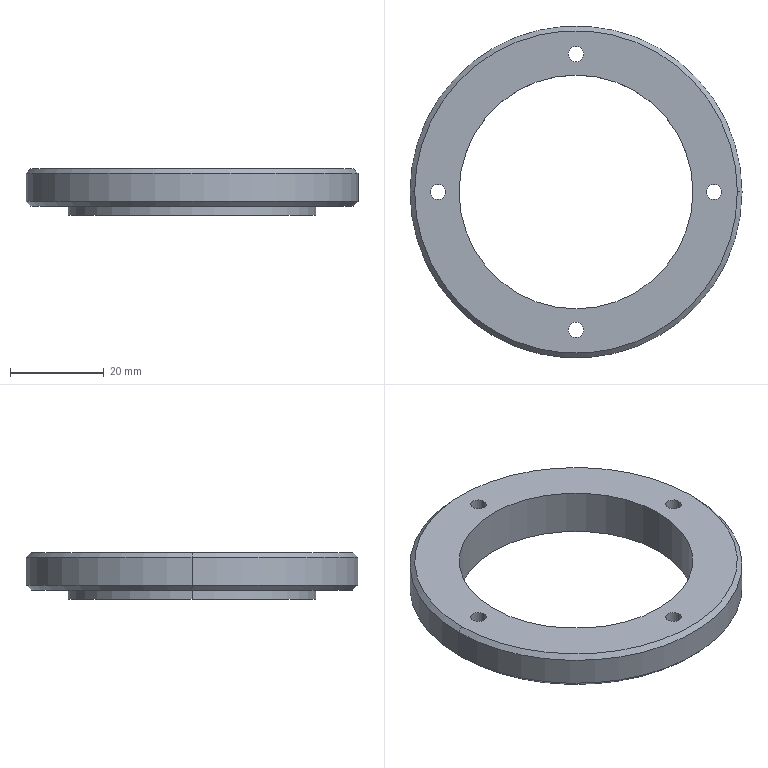Part | SolidWorks | features ICE 2, Chamfer 1, Extrusion 1, HoleWzd 1 | 1 solid | 21 faces | box 71 x 71 x 10 mm | volume 15956 mm3 | cylinder 14 | cone 4 | plane 3 | commonest cylinder face diameters 3.3 x8 50 x2 53 x2 71 x2
STEP:
#1=CARTESIAN_POINT('',(34.5,0.,10.));
#2=VERTEX_POINT('',#1);
#3=CARTESIAN_POINT('',(-34.5,0.,10.));
#4=VERTEX_POINT('',#3);
#5=CARTESIAN_POINT('',(0.,0.,10.));
#6=DIRECTION('',(0.,0.,1.));
#7=DIRECTION('',(1.,0.,0.));
#8=AXIS2_PLACEMENT_3D('',#5,#6,#7);
#9=CIRCLE('',#8,34.5);
#10=EDGE_CURVE('',#2,#4,#9,.T.);
#11=ORIENTED_EDGE('',*,*,#10,.F.);
#12=CARTESIAN_POINT('',(35.5,0.,9.));
#13=VERTEX_POINT('',#12);
#14=CARTESIAN_POINT('',(34.5,0.,10.));
#15=DIRECTION('',(0.7071,0.,-0.7071));
#16=VECTOR('',#15,1000.);
#17=LINE('',#14,#16);
#18=EDGE_CURVE('',#2,#13,#17,.T.);
#19=ORIENTED_EDGE('',*,*,#18,.T.);
#20=CARTESIAN_POINT('',(-35.5,0.,9.));
#21=VERTEX_POINT('',#20);
#22=CARTESIAN_POINT('',(0.,0.,9.));
#23=DIRECTION('',(0.,0.,-1.));
#24=DIRECTION('',(1.,0.,0.));
#25=AXIS2_PLACEMENT_3D('',#22,#23,#24);
#26=CIRCLE('',#25,35.5);
#27=EDGE_CURVE('',#21,#13,#26,.T.);
#28=ORIENTED_EDGE('',*,*,#27,.F.);
#29=CARTESIAN_POINT('',(-34.5,0.,10.));
#30=DIRECTION('',(-0.7071,0.,-0.7071));
#31=VECTOR('',#30,1000.);
#32=LINE('',#29,#31);
#33=EDGE_CURVE('',#4,#21,#32,.T.);
#34=ORIENTED_EDGE('',*,*,#33,.F.);
#35=EDGE_LOOP('',(#11,#19,#28,#34));
#36=FACE_OUTER_BOUND('',#35,.T.);
#37=CARTESIAN_POINT('',(0.,0.,10.));
#38=DIRECTION('',(0.,0.,-1.));
#39=DIRECTION('',(-1.,0.,0.));
#40=AXIS2_PLACEMENT_3D('',#37,#38,#39);
#41=CONICAL_SURFACE('',#40,34.5,0.7854);
#42=ADVANCED_FACE('',(#36),#41,.T.);
#43=CARTESIAN_POINT('',(-34.5,0.,2.));
#44=VERTEX_POINT('',#43);
#45=CARTESIAN_POINT('',(34.5,0.,2.));
#46=VERTEX_POINT('',#45);
#47=CARTESIAN_POINT('',(0.,0.,2.));
#48=DIRECTION('',(0.,0.,-1.));
#49=DIRECTION('',(-1.,0.,0.));
#50=AXIS2_PLACEMENT_3D('',#47,#48,#49);
#51=CIRCLE('',#50,34.5);
#52=EDGE_CURVE('',#44,#46,#51,.T.);
#53=ORIENTED_EDGE('',*,*,#52,.F.);
#54=CARTESIAN_POINT('',(-35.5,0.,3.));
#55=VERTEX_POINT('',#54);
#56=CARTESIAN_POINT('',(-34.5,0.,2.));
#57=DIRECTION('',(-0.7071,0.,0.7071));
#58=VECTOR('',#57,1000.);
#59=LINE('',#56,#58);
#60=EDGE_CURVE('',#44,#55,#59,.T.);
#61=ORIENTED_EDGE('',*,*,#60,.T.);
#62=CARTESIAN_POINT('',(35.5,0.,3.));
#63=VERTEX_POINT('',#62);
#64=CARTESIAN_POINT('',(0.,0.,3.));
#65=DIRECTION('',(0.,0.,1.));
#66=DIRECTION('',(-1.,0.,0.));
#67=AXIS2_PLACEMENT_3D('',#64,#65,#66);
#68=CIRCLE('',#67,35.5);
#69=EDGE_CURVE('',#63,#55,#68,.T.);
#70=ORIENTED_EDGE('',*,*,#69,.F.);
#71=CARTESIAN_POINT('',(34.5,0.,2.));
#72=DIRECTION('',(0.7071,0.,0.7071));
#73=VECTOR('',#72,1000.);
#74=LINE('',#71,#73);
#75=EDGE_CURVE('',#46,#63,#74,.T.);
#76=ORIENTED_EDGE('',*,*,#75,.F.);
#77=EDGE_LOOP('',(#53,#61,#70,#76));
#78=FACE_OUTER_BOUND('',#77,.T.);
#79=CARTESIAN_POINT('',(0.,0.,2.));
#80=DIRECTION('',(0.,0.,1.));
#81=DIRECTION('',(1.,0.,0.));
#82=AXIS2_PLACEMENT_3D('',#79,#80,#81);
#83=CONICAL_SURFACE('',#82,34.5,0.7854);
#84=ADVANCED_FACE('',(#78),#83,.T.);
#85=CARTESIAN_POINT('',(1.65,-29.5,2.));
#86=VERTEX_POINT('',#85);
#87=CARTESIAN_POINT('',(-1.65,-29.5,2.));
#88=VERTEX_POINT('',#87);
#89=CARTESIAN_POINT('',(0.,-29.5,2.));
#90=DIRECTION('',(0.,0.,-1.));
#91=DIRECTION('',(-1.,0.,0.));
#92=AXIS2_PLACEMENT_3D('',#89,#90,#91);
#93=CIRCLE('',#92,1.65);
#94=EDGE_CURVE('',#86,#88,#93,.T.);
#95=ORIENTED_EDGE('',*,*,#94,.T.);
#96=CARTESIAN_POINT('',(-1.65,-29.5,10.));
#97=VERTEX_POINT('',#96);
#98=CARTESIAN_POINT('',(-1.65,-29.5,10.));
#99=DIRECTION('',(0.,0.,1.));
#100=VECTOR('',#99,1000.);
#101=LINE('',#98,#100);
#102=EDGE_CURVE('',#88,#97,#101,.T.);
#103=ORIENTED_EDGE('',*,*,#102,.T.);
#104=CARTESIAN_POINT('',(1.65,-29.5,10.));
#105=VERTEX_POINT('',#104);
#106=CARTESIAN_POINT('',(0.,-29.5,10.));
#107=DIRECTION('',(0.,0.,1.));
#108=DIRECTION('',(1.,0.,0.));
#109=AXIS2_PLACEMENT_3D('',#106,#107,#108);
#110=CIRCLE('',#109,1.65);
#111=EDGE_CURVE('',#97,#105,#110,.T.);
#112=ORIENTED_EDGE('',*,*,#111,.T.);
#113=CARTESIAN_POINT('',(1.65,-29.5,10.));
#114=DIRECTION('',(0.,0.,1.));
#115=VECTOR('',#114,1000.);
#116=LINE('',#113,#115);
#117=EDGE_CURVE('',#86,#105,#116,.T.);
#118=ORIENTED_EDGE('',*,*,#117,.F.);
#119=EDGE_LOOP('',(#95,#103,#112,#118));
#120=FACE_OUTER_BOUND('',#119,.T.);
#121=CARTESIAN_POINT('',(0.,-29.5,10.));
#122=DIRECTION('',(0.,0.,1.));
#123=DIRECTION('',(1.,0.,0.));
#124=AXIS2_PLACEMENT_3D('',#121,#122,#123);
#125=CYLINDRICAL_SURFACE('',#124,1.65);
#126=ADVANCED_FACE('',(#120),#125,.F.);
#127=CARTESIAN_POINT('',(-27.85,0.,2.));
#128=VERTEX_POINT('',#127);
#129=CARTESIAN_POINT('',(-31.15,0.,2.));
#130=VERTEX_POINT('',#129);
#131=CARTESIAN_POINT('',(-29.5,0.,2.));
#132=DIRECTION('',(0.,0.,-1.));
#133=DIRECTION('',(-1.,0.,0.));
#134=AXIS2_PLACEMENT_3D('',#131,#132,#133);
#135=CIRCLE('',#134,1.65);
#136=EDGE_CURVE('',#128,#130,#135,.T.);
#137=ORIENTED_EDGE('',*,*,#136,.T.);
#138=CARTESIAN_POINT('',(-31.15,0.,10.));
#139=VERTEX_POINT('',#138);
#140=CARTESIAN_POINT('',(-31.15,0.,10.));
#141=DIRECTION('',(0.,0.,1.));
#142=VECTOR('',#141,1000.);
#143=LINE('',#140,#142);
#144=EDGE_CURVE('',#130,#139,#143,.T.);
#145=ORIENTED_EDGE('',*,*,#144,.T.);
#146=CARTESIAN_POINT('',(-27.85,0.,10.));
#147=VERTEX_POINT('',#146);
#148=CARTESIAN_POINT('',(-29.5,0.,10.));
#149=DIRECTION('',(0.,0.,1.));
#150=DIRECTION('',(1.,0.,0.));
#151=AXIS2_PLACEMENT_3D('',#148,#149,#150);
#152=CIRCLE('',#151,1.65);
#153=EDGE_CURVE('',#139,#147,#152,.T.);
#154=ORIENTED_EDGE('',*,*,#153,.T.);
#155=CARTESIAN_POINT('',(-27.85,0.,10.));
#156=DIRECTION('',(0.,0.,1.));
#157=VECTOR('',#156,1000.);
#158=LINE('',#155,#157);
#159=EDGE_CURVE('',#128,#147,#158,.T.);
#160=ORIENTED_EDGE('',*,*,#159,.F.);
#161=EDGE_LOOP('',(#137,#145,#154,#160));
#162=FACE_OUTER_BOUND('',#161,.T.);
#163=CARTESIAN_POINT('',(-29.5,0.,10.));
#164=DIRECTION('',(0.,0.,1.));
#165=DIRECTION('',(1.,0.,0.));
#166=AXIS2_PLACEMENT_3D('',#163,#164,#165);
#167=CYLINDRICAL_SURFACE('',#166,1.65);
#168=ADVANCED_FACE('',(#162),#167,.F.);
#169=CARTESIAN_POINT('',(1.65,29.5,2.));
#170=VERTEX_POINT('',#169);
#171=CARTESIAN_POINT('',(-1.65,29.5,2.));
#172=VERTEX_POINT('',#171);
#173=CARTESIAN_POINT('',(0.,29.5,2.));
#174=DIRECTION('',(0.,0.,-1.));
#175=DIRECTION('',(-1.,0.,0.));
#176=AXIS2_PLACEMENT_3D('',#173,#174,#175);
#177=CIRCLE('',#176,1.65);
#178=EDGE_CURVE('',#170,#172,#177,.T.);
#179=ORIENTED_EDGE('',*,*,#178,.T.);
#180=CARTESIAN_POINT('',(-1.65,29.5,10.));
#181=VERTEX_POINT('',#180);
#182=CARTESIAN_POINT('',(-1.65,29.5,10.));
#183=DIRECTION('',(0.,0.,1.));
#184=VECTOR('',#183,1000.);
#185=LINE('',#182,#184);
#186=EDGE_CURVE('',#172,#181,#185,.T.);
#187=ORIENTED_EDGE('',*,*,#186,.T.);
#188=CARTESIAN_POINT('',(1.65,29.5,10.));
#189=VERTEX_POINT('',#188);
#190=CARTESIAN_POINT('',(0.,29.5,10.));
#191=DIRECTION('',(0.,0.,1.));
#192=DIRECTION('',(1.,0.,0.));
#193=AXIS2_PLACEMENT_3D('',#190,#191,#192);
#194=CIRCLE('',#193,1.65);
#195=EDGE_CURVE('',#181,#189,#194,.T.);
#196=ORIENTED_EDGE('',*,*,#195,.T.);
#197=CARTESIAN_POINT('',(1.65,29.5,10.));
#198=DIRECTION('',(0.,0.,1.));
#199=VECTOR('',#198,1000.);
#200=LINE('',#197,#199);
#201=EDGE_CURVE('',#170,#189,#200,.T.);
#202=ORIENTED_EDGE('',*,*,#201,.F.);
#203=EDGE_LOOP('',(#179,#187,#196,#202));
#204=FACE_OUTER_BOUND('',#203,.T.);
#205=CARTESIAN_POINT('',(0.,29.5,10.));
#206=DIRECTION('',(0.,0.,1.));
#207=DIRECTION('',(1.,0.,0.));
#208=AXIS2_PLACEMENT_3D('',#205,#206,#207);
#209=CYLINDRICAL_SURFACE('',#208,1.65);
#210=ADVANCED_FACE('',(#204),#209,.F.);
#211=CARTESIAN_POINT('',(31.15,0.,2.));
#212=VERTEX_POINT('',#211);
#213=CARTESIAN_POINT('',(27.85,0.,2.));
#214=VERTEX_POINT('',#213);
#215=CARTESIAN_POINT('',(29.5,0.,2.));
#216=DIRECTION('',(0.,0.,-1.));
#217=DIRECTION('',(-1.,0.,0.));
#218=AXIS2_PLACEMENT_3D('',#215,#216,#217);
#219=CIRCLE('',#218,1.65);
#220=EDGE_CURVE('',#212,#214,#219,.T.);
#221=ORIENTED_EDGE('',*,*,#220,.T.);
#222=CARTESIAN_POINT('',(27.85,0.,10.));
#223=VERTEX_POINT('',#222);
#224=CARTESIAN_POINT('',(27.85,0.,10.));
#225=DIRECTION('',(0.,0.,1.));
#226=VECTOR('',#225,1000.);
#227=LINE('',#224,#226);
#228=EDGE_CURVE('',#214,#223,#227,.T.);
#229=ORIENTED_EDGE('',*,*,#228,.T.);
#230=CARTESIAN_POINT('',(31.15,0.,10.));
#231=VERTEX_POINT('',#230);
#232=CARTESIAN_POINT('',(29.5,0.,10.));
#233=DIRECTION('',(0.,0.,1.));
#234=DIRECTION('',(1.,0.,0.));
#235=AXIS2_PLACEMENT_3D('',#232,#233,#234);
#236=CIRCLE('',#235,1.65);
#237=EDGE_CURVE('',#223,#231,#236,.T.);
#238=ORIENTED_EDGE('',*,*,#237,.T.);
#239=CARTESIAN_POINT('',(31.15,0.,10.));
#240=DIRECTION('',(0.,0.,1.));
#241=VECTOR('',#240,1000.);
#242=LINE('',#239,#241);
#243=EDGE_CURVE('',#212,#231,#242,.T.);
#244=ORIENTED_EDGE('',*,*,#243,.F.);
#245=EDGE_LOOP('',(#221,#229,#238,#244));
#246=FACE_OUTER_BOUND('',#245,.T.);
#247=CARTESIAN_POINT('',(29.5,0.,10.));
#248=DIRECTION('',(0.,0.,1.));
#249=DIRECTION('',(1.,0.,0.));
#250=AXIS2_PLACEMENT_3D('',#247,#248,#249);
#251=CYLINDRICAL_SURFACE('',#250,1.65);
#252=ADVANCED_FACE('',(#246),#251,.F.);
#253=CARTESIAN_POINT('',(-26.5,0.,2.));
#254=VERTEX_POINT('',#253);
#255=CARTESIAN_POINT('',(26.5,0.,2.));
#256=VERTEX_POINT('',#255);
#257=CARTESIAN_POINT('',(0.,0.,2.));
#258=DIRECTION('',(0.,0.,-1.));
#259=DIRECTION('',(-1.,0.,0.));
#260=AXIS2_PLACEMENT_3D('',#257,#258,#259);
#261=CIRCLE('',#260,26.5);
#262=EDGE_CURVE('',#254,#256,#261,.T.);
#263=ORIENTED_EDGE('',*,*,#262,.T.);
#264=CARTESIAN_POINT('',(26.5,0.,0.));
#265=VERTEX_POINT('',#264);
#266=CARTESIAN_POINT('',(26.5,0.,2.));
#267=DIRECTION('',(0.,0.,-1.));
#268=VECTOR('',#267,1000.);
#269=LINE('',#266,#268);
#270=EDGE_CURVE('',#256,#265,#269,.T.);
#271=ORIENTED_EDGE('',*,*,#270,.T.);
#272=CARTESIAN_POINT('',(-26.5,0.,0.));
#273=VERTEX_POINT('',#272);
#274=CARTESIAN_POINT('',(0.,0.,0.));
#275=DIRECTION('',(0.,0.,-1.));
#276=DIRECTION('',(-1.,0.,0.));
#277=AXIS2_PLACEMENT_3D('',#274,#275,#276);
#278=CIRCLE('',#277,26.5);
#279=EDGE_CURVE('',#273,#265,#278,.T.);
#280=ORIENTED_EDGE('',*,*,#279,.F.);
#281=CARTESIAN_POINT('',(-26.5,0.,2.));
#282=DIRECTION('',(0.,0.,-1.));
#283=VECTOR('',#282,1000.);
#284=LINE('',#281,#283);
#285=EDGE_CURVE('',#254,#273,#284,.T.);
#286=ORIENTED_EDGE('',*,*,#285,.F.);
#287=EDGE_LOOP('',(#263,#271,#280,#286));
#288=FACE_OUTER_BOUND('',#287,.T.);
#289=CARTESIAN_POINT('',(0.,0.,2.));
#290=DIRECTION('',(0.,0.,-1.));
#291=DIRECTION('',(-1.,0.,0.));
#292=AXIS2_PLACEMENT_3D('',#289,#290,#291);
#293=CYLINDRICAL_SURFACE('',#292,26.5);
#294=ADVANCED_FACE('',(#288),#293,.T.);
#295=CARTESIAN_POINT('',(-25.,0.,10.));
#296=VERTEX_POINT('',#295);
#297=CARTESIAN_POINT('',(25.,0.,10.));
#298=VERTEX_POINT('',#297);
#299=CARTESIAN_POINT('',(0.,0.,10.));
#300=DIRECTION('',(0.,0.,1.));
#301=DIRECTION('',(1.,0.,0.));
#302=AXIS2_PLACEMENT_3D('',#299,#300,#301);
#303=CIRCLE('',#302,25.);
#304=EDGE_CURVE('',#296,#298,#303,.T.);
#305=ORIENTED_EDGE('',*,*,#304,.T.);
#306=CARTESIAN_POINT('',(25.,0.,0.));
#307=VERTEX_POINT('',#306);
#308=CARTESIAN_POINT('',(25.,0.,10.));
#309=DIRECTION('',(0.,0.,-1.));
#310=VECTOR('',#309,1000.);
#311=LINE('',#308,#310);
#312=EDGE_CURVE('',#298,#307,#311,.T.);
#313=ORIENTED_EDGE('',*,*,#312,.T.);
#314=CARTESIAN_POINT('',(-25.,0.,0.));
#315=VERTEX_POINT('',#314);
#316=CARTESIAN_POINT('',(0.,0.,0.));
#317=DIRECTION('',(0.,0.,1.));
#318=DIRECTION('',(1.,0.,0.));
#319=AXIS2_PLACEMENT_3D('',#316,#317,#318);
#320=CIRCLE('',#319,25.);
#321=EDGE_CURVE('',#315,#307,#320,.T.);
#322=ORIENTED_EDGE('',*,*,#321,.F.);
#323=CARTESIAN_POINT('',(-25.,0.,10.));
#324=DIRECTION('',(0.,0.,-1.));
#325=VECTOR('',#324,1000.);
#326=LINE('',#323,#325);
#327=EDGE_CURVE('',#296,#315,#326,.T.);
#328=ORIENTED_EDGE('',*,*,#327,.F.);
#329=EDGE_LOOP('',(#305,#313,#322,#328));
#330=FACE_OUTER_BOUND('',#329,.T.);
#331=CARTESIAN_POINT('',(0.,0.,10.));
#332=DIRECTION('',(0.,0.,-1.));
#333=DIRECTION('',(-1.,0.,0.));
#334=AXIS2_PLACEMENT_3D('',#331,#332,#333);
#335=CYLINDRICAL_SURFACE('',#334,25.);
#336=ADVANCED_FACE('',(#330),#335,.F.);
#337=ORIENTED_EDGE('',*,*,#27,.T.);
#338=CARTESIAN_POINT('',(35.5,0.,10.));
#339=DIRECTION('',(0.,0.,-1.));
#340=VECTOR('',#339,1000.);
#341=LINE('',#338,#340);
#342=EDGE_CURVE('',#13,#63,#341,.T.);
#343=ORIENTED_EDGE('',*,*,#342,.T.);
#344=ORIENTED_EDGE('',*,*,#69,.T.);
#345=CARTESIAN_POINT('',(-35.5,0.,10.));
#346=DIRECTION('',(0.,0.,-1.));
#347=VECTOR('',#346,1000.);
#348=LINE('',#345,#347);
#349=EDGE_CURVE('',#21,#55,#348,.T.);
#350=ORIENTED_EDGE('',*,*,#349,.F.);
#351=EDGE_LOOP('',(#337,#343,#344,#350));
#352=FACE_OUTER_BOUND('',#351,.T.);
#353=CARTESIAN_POINT('',(0.,0.,10.));
#354=DIRECTION('',(0.,0.,-1.));
#355=DIRECTION('',(-1.,0.,0.));
#356=AXIS2_PLACEMENT_3D('',#353,#354,#355);
#357=CYLINDRICAL_SURFACE('',#356,35.5);
#358=ADVANCED_FACE('',(#352),#357,.T.);
#359=ORIENTED_EDGE('',*,*,#321,.T.);
#360=CARTESIAN_POINT('',(0.,0.,0.));
#361=DIRECTION('',(0.,0.,1.));
#362=DIRECTION('',(1.,0.,0.));
#363=AXIS2_PLACEMENT_3D('',#360,#361,#362);
#364=CIRCLE('',#363,25.);
#365=EDGE_CURVE('',#307,#315,#364,.T.);
#366=ORIENTED_EDGE('',*,*,#365,.T.);
#367=EDGE_LOOP('',(#359,#366));
#368=FACE_BOUND('',#367,.T.);
#369=ORIENTED_EDGE('',*,*,#279,.T.);
#370=CARTESIAN_POINT('',(0.,0.,0.));
#371=DIRECTION('',(0.,0.,-1.));
#372=DIRECTION('',(-1.,0.,0.));
#373=AXIS2_PLACEMENT_3D('',#370,#371,#372);
#374=CIRCLE('',#373,26.5);
#375=EDGE_CURVE('',#265,#273,#374,.T.);
#376=ORIENTED_EDGE('',*,*,#375,.T.);
#377=EDGE_LOOP('',(#369,#376));
#378=FACE_OUTER_BOUND('',#377,.T.);
#379=CARTESIAN_POINT('',(0.,0.,0.));
#380=DIRECTION('',(0.,0.,1.));
#381=DIRECTION('',(1.,0.,0.));
#382=AXIS2_PLACEMENT_3D('',#379,#380,#381);
#383=PLANE('',#382);
#384=ADVANCED_FACE('',(#368,#378),#383,.F.);
#385=ORIENTED_EDGE('',*,*,#342,.F.);
#386=CARTESIAN_POINT('',(0.,0.,9.));
#387=DIRECTION('',(0.,0.,-1.));
#388=DIRECTION('',(1.,0.,0.));
#389=AXIS2_PLACEMENT_3D('',#386,#387,#388);
#390=CIRCLE('',#389,35.5);
#391=EDGE_CURVE('',#13,#21,#390,.T.);
#392=ORIENTED_EDGE('',*,*,#391,.T.);
#393=ORIENTED_EDGE('',*,*,#349,.T.);
#394=CARTESIAN_POINT('',(0.,0.,3.));
#395=DIRECTION('',(0.,0.,1.));
#396=DIRECTION('',(-1.,0.,0.));
#397=AXIS2_PLACEMENT_3D('',#394,#395,#396);
#398=CIRCLE('',#397,35.5);
#399=EDGE_CURVE('',#55,#63,#398,.T.);
#400=ORIENTED_EDGE('',*,*,#399,.T.);
#401=EDGE_LOOP('',(#385,#392,#393,#400));
#402=FACE_OUTER_BOUND('',#401,.T.);
#403=CARTESIAN_POINT('',(0.,0.,10.));
#404=DIRECTION('',(0.,0.,-1.));
#405=DIRECTION('',(-1.,0.,0.));
#406=AXIS2_PLACEMENT_3D('',#403,#404,#405);
#407=CYLINDRICAL_SURFACE('',#406,35.5);
#408=ADVANCED_FACE('',(#402),#407,.T.);
#409=CARTESIAN_POINT('',(0.,0.,10.));
#410=DIRECTION('',(0.,0.,1.));
#411=DIRECTION('',(1.,0.,0.));
#412=AXIS2_PLACEMENT_3D('',#409,#410,#411);
#413=CIRCLE('',#412,34.5);
#414=EDGE_CURVE('',#4,#2,#413,.T.);
#415=ORIENTED_EDGE('',*,*,#414,.T.);
#416=ORIENTED_EDGE('',*,*,#10,.T.);
#417=EDGE_LOOP('',(#415,#416));
#418=FACE_OUTER_BOUND('',#417,.T.);
#419=CARTESIAN_POINT('',(0.,-29.5,10.));
#420=DIRECTION('',(0.,0.,1.));
#421=DIRECTION('',(1.,0.,0.));
#422=AXIS2_PLACEMENT_3D('',#419,#420,#421);
#423=CIRCLE('',#422,1.65);
#424=EDGE_CURVE('',#105,#97,#423,.T.);
#425=ORIENTED_EDGE('',*,*,#424,.F.);
#426=ORIENTED_EDGE('',*,*,#111,.F.);
#427=EDGE_LOOP('',(#425,#426));
#428=FACE_BOUND('',#427,.T.);
#429=CARTESIAN_POINT('',(-29.5,0.,10.));
#430=DIRECTION('',(0.,0.,1.));
#431=DIRECTION('',(1.,0.,0.));
#432=AXIS2_PLACEMENT_3D('',#429,#430,#431);
#433=CIRCLE('',#432,1.65);
#434=EDGE_CURVE('',#147,#139,#433,.T.);
#435=ORIENTED_EDGE('',*,*,#434,.F.);
#436=ORIENTED_EDGE('',*,*,#153,.F.);
#437=EDGE_LOOP('',(#435,#436));
#438=FACE_BOUND('',#437,.T.);
#439=CARTESIAN_POINT('',(0.,29.5,10.));
#440=DIRECTION('',(0.,0.,1.));
#441=DIRECTION('',(1.,0.,0.));
#442=AXIS2_PLACEMENT_3D('',#439,#440,#441);
#443=CIRCLE('',#442,1.65);
#444=EDGE_CURVE('',#189,#181,#443,.T.);
#445=ORIENTED_EDGE('',*,*,#444,.F.);
#446=ORIENTED_EDGE('',*,*,#195,.F.);
#447=EDGE_LOOP('',(#445,#446));
#448=FACE_BOUND('',#447,.T.);
#449=CARTESIAN_POINT('',(29.5,0.,10.));
#450=DIRECTION('',(0.,0.,1.));
#451=DIRECTION('',(1.,0.,0.));
#452=AXIS2_PLACEMENT_3D('',#449,#450,#451);
#453=CIRCLE('',#452,1.65);
#454=EDGE_CURVE('',#231,#223,#453,.T.);
#455=ORIENTED_EDGE('',*,*,#454,.F.);
#456=ORIENTED_EDGE('',*,*,#237,.F.);
#457=EDGE_LOOP('',(#455,#456));
#458=FACE_BOUND('',#457,.T.);
#459=ORIENTED_EDGE('',*,*,#304,.F.);
#460=CARTESIAN_POINT('',(0.,0.,10.));
#461=DIRECTION('',(0.,0.,1.));
#462=DIRECTION('',(1.,0.,0.));
#463=AXIS2_PLACEMENT_3D('',#460,#461,#462);
#464=CIRCLE('',#463,25.);
#465=EDGE_CURVE('',#298,#296,#464,.T.);
#466=ORIENTED_EDGE('',*,*,#465,.F.);
#467=EDGE_LOOP('',(#459,#466));
#468=FACE_BOUND('',#467,.T.);
#469=CARTESIAN_POINT('',(0.,0.,10.));
#470=DIRECTION('',(0.,0.,1.));
#471=DIRECTION('',(1.,0.,0.));
#472=AXIS2_PLACEMENT_3D('',#469,#470,#471);
#473=PLANE('',#472);
#474=ADVANCED_FACE('',(#418,#428,#438,#448,#458,#468),#473,.T.);
#475=ORIENTED_EDGE('',*,*,#312,.F.);
#476=ORIENTED_EDGE('',*,*,#465,.T.);
#477=ORIENTED_EDGE('',*,*,#327,.T.);
#478=ORIENTED_EDGE('',*,*,#365,.F.);
#479=EDGE_LOOP('',(#475,#476,#477,#478));
#480=FACE_OUTER_BOUND('',#479,.T.);
#481=CARTESIAN_POINT('',(0.,0.,10.));
#482=DIRECTION('',(0.,0.,-1.));
#483=DIRECTION('',(-1.,0.,0.));
#484=AXIS2_PLACEMENT_3D('',#481,#482,#483);
#485=CYLINDRICAL_SURFACE('',#484,25.);
#486=ADVANCED_FACE('',(#480),#485,.F.);
#487=CARTESIAN_POINT('',(0.,0.,2.));
#488=DIRECTION('',(0.,0.,-1.));
#489=DIRECTION('',(-1.,0.,0.));
#490=AXIS2_PLACEMENT_3D('',#487,#488,#489);
#491=CIRCLE('',#490,34.5);
#492=EDGE_CURVE('',#46,#44,#491,.T.);
#493=ORIENTED_EDGE('',*,*,#492,.T.);
#494=ORIENTED_EDGE('',*,*,#52,.T.);
#495=EDGE_LOOP('',(#493,#494));
#496=FACE_OUTER_BOUND('',#495,.T.);
#497=ORIENTED_EDGE('',*,*,#94,.F.);
#498=CARTESIAN_POINT('',(0.,-29.5,2.));
#499=DIRECTION('',(0.,0.,-1.));
#500=DIRECTION('',(-1.,0.,0.));
#501=AXIS2_PLACEMENT_3D('',#498,#499,#500);
#502=CIRCLE('',#501,1.65);
#503=EDGE_CURVE('',#88,#86,#502,.T.);
#504=ORIENTED_EDGE('',*,*,#503,.F.);
#505=EDGE_LOOP('',(#497,#504));
#506=FACE_BOUND('',#505,.T.);
#507=ORIENTED_EDGE('',*,*,#136,.F.);
#508=CARTESIAN_POINT('',(-29.5,0.,2.));
#509=DIRECTION('',(0.,0.,-1.));
#510=DIRECTION('',(-1.,0.,0.));
#511=AXIS2_PLACEMENT_3D('',#508,#509,#510);
#512=CIRCLE('',#511,1.65);
#513=EDGE_CURVE('',#130,#128,#512,.T.);
#514=ORIENTED_EDGE('',*,*,#513,.F.);
#515=EDGE_LOOP('',(#507,#514));
#516=FACE_BOUND('',#515,.T.);
#517=ORIENTED_EDGE('',*,*,#178,.F.);
#518=CARTESIAN_POINT('',(0.,29.5,2.));
#519=DIRECTION('',(0.,0.,-1.));
#520=DIRECTION('',(-1.,0.,0.));
#521=AXIS2_PLACEMENT_3D('',#518,#519,#520);
#522=CIRCLE('',#521,1.65);
#523=EDGE_CURVE('',#172,#170,#522,.T.);
#524=ORIENTED_EDGE('',*,*,#523,.F.);
#525=EDGE_LOOP('',(#517,#524));
#526=FACE_BOUND('',#525,.T.);
#527=ORIENTED_EDGE('',*,*,#220,.F.);
#528=CARTESIAN_POINT('',(29.5,0.,2.));
#529=DIRECTION('',(0.,0.,-1.));
#530=DIRECTION('',(-1.,0.,0.));
#531=AXIS2_PLACEMENT_3D('',#528,#529,#530);
#532=CIRCLE('',#531,1.65);
#533=EDGE_CURVE('',#214,#212,#532,.T.);
#534=ORIENTED_EDGE('',*,*,#533,.F.);
#535=EDGE_LOOP('',(#527,#534));
#536=FACE_BOUND('',#535,.T.);
#537=ORIENTED_EDGE('',*,*,#262,.F.);
#538=CARTESIAN_POINT('',(0.,0.,2.));
#539=DIRECTION('',(0.,0.,-1.));
#540=DIRECTION('',(-1.,0.,0.));
#541=AXIS2_PLACEMENT_3D('',#538,#539,#540);
#542=CIRCLE('',#541,26.5);
#543=EDGE_CURVE('',#256,#254,#542,.T.);
#544=ORIENTED_EDGE('',*,*,#543,.F.);
#545=EDGE_LOOP('',(#537,#544));
#546=FACE_BOUND('',#545,.T.);
#547=CARTESIAN_POINT('',(0.,0.,2.));
#548=DIRECTION('',(0.,0.,-1.));
#549=DIRECTION('',(-1.,0.,0.));
#550=AXIS2_PLACEMENT_3D('',#547,#548,#549);
#551=PLANE('',#550);
#552=ADVANCED_FACE('',(#496,#506,#516,#526,#536,#546),#551,.T.);
#553=ORIENTED_EDGE('',*,*,#270,.F.);
#554=ORIENTED_EDGE('',*,*,#543,.T.);
#555=ORIENTED_EDGE('',*,*,#285,.T.);
#556=ORIENTED_EDGE('',*,*,#375,.F.);
#557=EDGE_LOOP('',(#553,#554,#555,#556));
#558=FACE_OUTER_BOUND('',#557,.T.);
#559=CARTESIAN_POINT('',(0.,0.,2.));
#560=DIRECTION('',(0.,0.,-1.));
#561=DIRECTION('',(-1.,0.,0.));
#562=AXIS2_PLACEMENT_3D('',#559,#560,#561);
#563=CYLINDRICAL_SURFACE('',#562,26.5);
#564=ADVANCED_FACE('',(#558),#563,.T.);
#565=ORIENTED_EDGE('',*,*,#228,.F.);
#566=ORIENTED_EDGE('',*,*,#533,.T.);
#567=ORIENTED_EDGE('',*,*,#243,.T.);
#568=ORIENTED_EDGE('',*,*,#454,.T.);
#569=EDGE_LOOP('',(#565,#566,#567,#568));
#570=FACE_OUTER_BOUND('',#569,.T.);
#571=CARTESIAN_POINT('',(29.5,0.,10.));
#572=DIRECTION('',(0.,0.,1.));
#573=DIRECTION('',(1.,0.,0.));
#574=AXIS2_PLACEMENT_3D('',#571,#572,#573);
#575=CYLINDRICAL_SURFACE('',#574,1.65);
#576=ADVANCED_FACE('',(#570),#575,.F.);
#577=ORIENTED_EDGE('',*,*,#186,.F.);
#578=ORIENTED_EDGE('',*,*,#523,.T.);
#579=ORIENTED_EDGE('',*,*,#201,.T.);
#580=ORIENTED_EDGE('',*,*,#444,.T.);
#581=EDGE_LOOP('',(#577,#578,#579,#580));
#582=FACE_OUTER_BOUND('',#581,.T.);
#583=CARTESIAN_POINT('',(0.,29.5,10.));
#584=DIRECTION('',(0.,0.,1.));
#585=DIRECTION('',(1.,0.,0.));
#586=AXIS2_PLACEMENT_3D('',#583,#584,#585);
#587=CYLINDRICAL_SURFACE('',#586,1.65);
#588=ADVANCED_FACE('',(#582),#587,.F.);
#589=ORIENTED_EDGE('',*,*,#144,.F.);
#590=ORIENTED_EDGE('',*,*,#513,.T.);
#591=ORIENTED_EDGE('',*,*,#159,.T.);
#592=ORIENTED_EDGE('',*,*,#434,.T.);
#593=EDGE_LOOP('',(#589,#590,#591,#592));
#594=FACE_OUTER_BOUND('',#593,.T.);
#595=CARTESIAN_POINT('',(-29.5,0.,10.));
#596=DIRECTION('',(0.,0.,1.));
#597=DIRECTION('',(1.,0.,0.));
#598=AXIS2_PLACEMENT_3D('',#595,#596,#597);
#599=CYLINDRICAL_SURFACE('',#598,1.65);
#600=ADVANCED_FACE('',(#594),#599,.F.);
#601=ORIENTED_EDGE('',*,*,#102,.F.);
#602=ORIENTED_EDGE('',*,*,#503,.T.);
#603=ORIENTED_EDGE('',*,*,#117,.T.);
#604=ORIENTED_EDGE('',*,*,#424,.T.);
#605=EDGE_LOOP('',(#601,#602,#603,#604));
#606=FACE_OUTER_BOUND('',#605,.T.);
#607=CARTESIAN_POINT('',(0.,-29.5,10.));
#608=DIRECTION('',(0.,0.,1.));
#609=DIRECTION('',(1.,0.,0.));
#610=AXIS2_PLACEMENT_3D('',#607,#608,#609);
#611=CYLINDRICAL_SURFACE('',#610,1.65);
#612=ADVANCED_FACE('',(#606),#611,.F.);
#613=ORIENTED_EDGE('',*,*,#60,.F.);
#614=ORIENTED_EDGE('',*,*,#492,.F.);
#615=ORIENTED_EDGE('',*,*,#75,.T.);
#616=ORIENTED_EDGE('',*,*,#399,.F.);
#617=EDGE_LOOP('',(#613,#614,#615,#616));
#618=FACE_OUTER_BOUND('',#617,.T.);
#619=CARTESIAN_POINT('',(0.,0.,2.));
#620=DIRECTION('',(0.,0.,1.));
#621=DIRECTION('',(1.,0.,0.));
#622=AXIS2_PLACEMENT_3D('',#619,#620,#621);
#623=CONICAL_SURFACE('',#622,34.5,0.7854);
#624=ADVANCED_FACE('',(#618),#623,.T.);
#625=ORIENTED_EDGE('',*,*,#18,.F.);
#626=ORIENTED_EDGE('',*,*,#414,.F.);
#627=ORIENTED_EDGE('',*,*,#33,.T.);
#628=ORIENTED_EDGE('',*,*,#391,.F.);
#629=EDGE_LOOP('',(#625,#626,#627,#628));
#630=FACE_OUTER_BOUND('',#629,.T.);
#631=CARTESIAN_POINT('',(0.,0.,10.));
#632=DIRECTION('',(0.,0.,-1.));
#633=DIRECTION('',(-1.,0.,0.));
#634=AXIS2_PLACEMENT_3D('',#631,#632,#633);
#635=CONICAL_SURFACE('',#634,34.5,0.7854);
#636=ADVANCED_FACE('',(#630),#635,.T.);
#637=CLOSED_SHELL('',(#42,#84,#126,#168,#210,#252,#294,#336,#358,#384,#408,#474,#486,#552,#564,#576,#588,#600,#612,#624,#636));
#638=MANIFOLD_SOLID_BREP('',#637);
#639=CARTESIAN_POINT('',(0.,0.,0.));
#640=DIRECTION('',(0.,0.,1.));
#641=DIRECTION('',(1.,0.,0.));
#642=AXIS2_PLACEMENT_3D('',#639,#640,#641);
#643=(LENGTH_UNIT()NAMED_UNIT(*)SI_UNIT(.MILLI.,.METRE.));
#644=UNCERTAINTY_MEASURE_WITH_UNIT(LENGTH_MEASURE(0.00001),#643,'','');
#645=(NAMED_UNIT(*)PLANE_ANGLE_UNIT()SI_UNIT($,.RADIAN.));
#646=(NAMED_UNIT(*)SI_UNIT($,.STERADIAN.)SOLID_ANGLE_UNIT());
#647=(GEOMETRIC_REPRESENTATION_CONTEXT(3)GLOBAL_UNCERTAINTY_ASSIGNED_CONTEXT((#644))GLOBAL_UNIT_ASSIGNED_CONTEXT((#643,#645,#646))REPRESENTATION_CONTEXT('',''));
#648=ADVANCED_BREP_SHAPE_REPRESENTATION('',(#638,#642),#647);